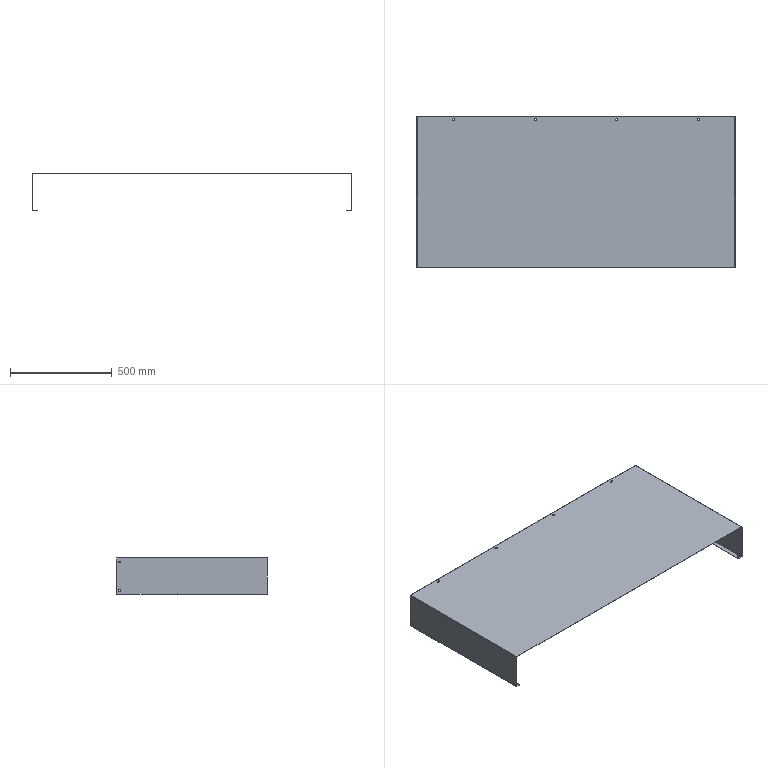Part | SolidWorks | features BaseBody 1 | 1 solid | 112 faces | box 1564 x 740 x 181.2 mm | volume 1730963 mm3 | plane 78 | cylinder 34 | commonest cylinder face diameters 7 x20 10 x6 2 x4 4.4 x4